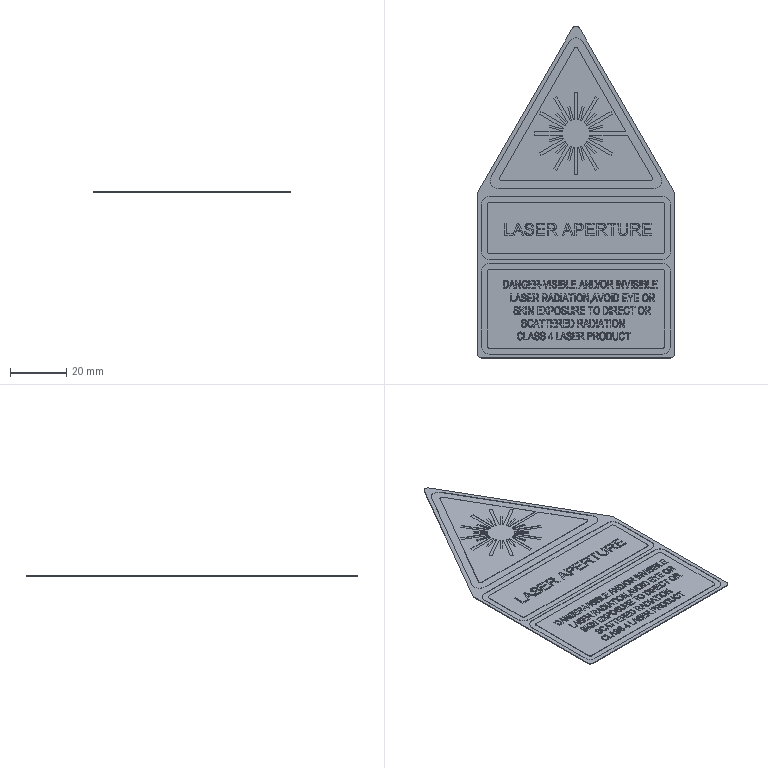Part | STEP file | BBS-JG-IEC-L70X118-1.stp.STEP | 1 solid | 2392 faces | box 70 x 118.022 x 0.28 mm | volume 1499 mm3 | plane 1204 | spline 1137 | cylinder 51 | commonest cylinder face diameters 9.8 x24 1.4 x11 5.6 x11 2.8 x5